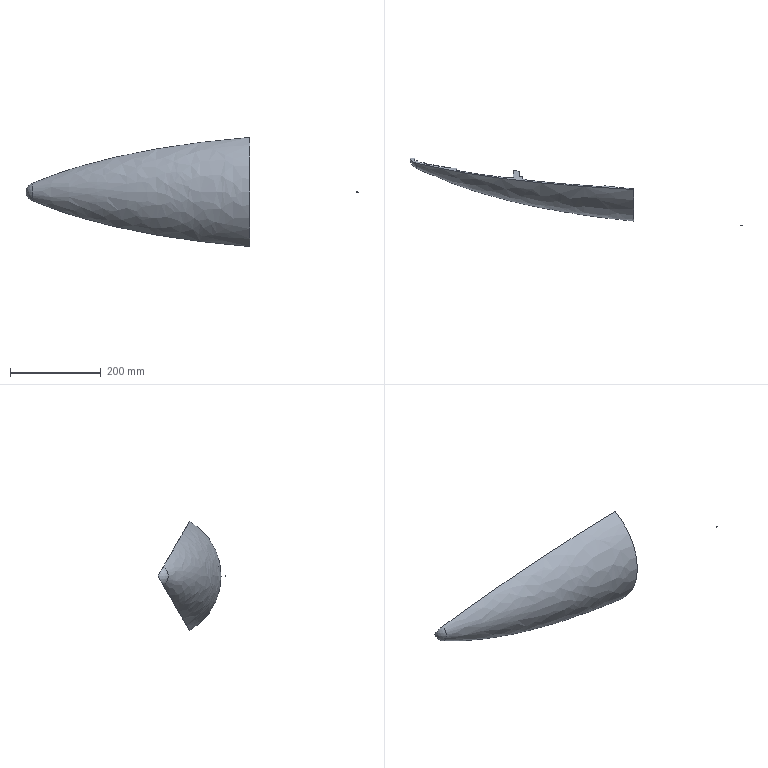Part | SolidWorks | features ICE 5, Fillet 3, Revolution 3, CombineBodies 1, RefAxis 1, RevCut 1 | 2 solids | 75 faces | box 733.25 x 150.001 x 241.12 mm | volume 643249 mm3 | plane 30 | cylinder 21 | cone 12 | spline 10 | sphere 1 | torus 1 | commonest cylinder face diameters 10 x4 6 x2 20 x2 25.446 x1 36.172 x1 41.974 x1